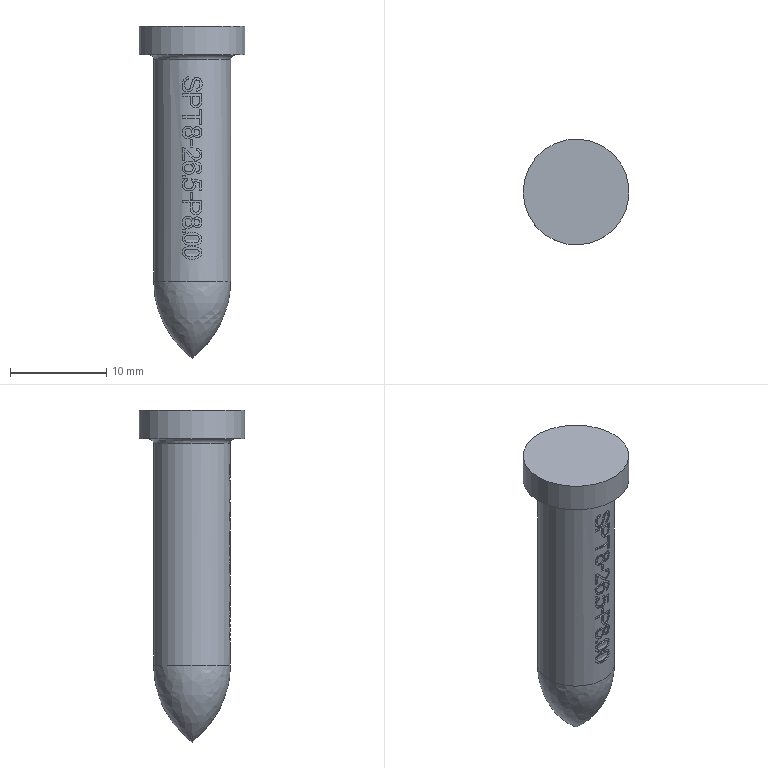Part | STEP file | PN_0063_id790_x_t | 1 solid | 194 faces | box 11 x 11 x 34.5 mm | volume 1696 mm3 | plane 101 | cylinder 91 | torus 1 | spline 1 | commonest cylinder face diameters 7.8 x15 8 x10 0.645 x4 0.806 x4 1.154 x3 0.711 x2